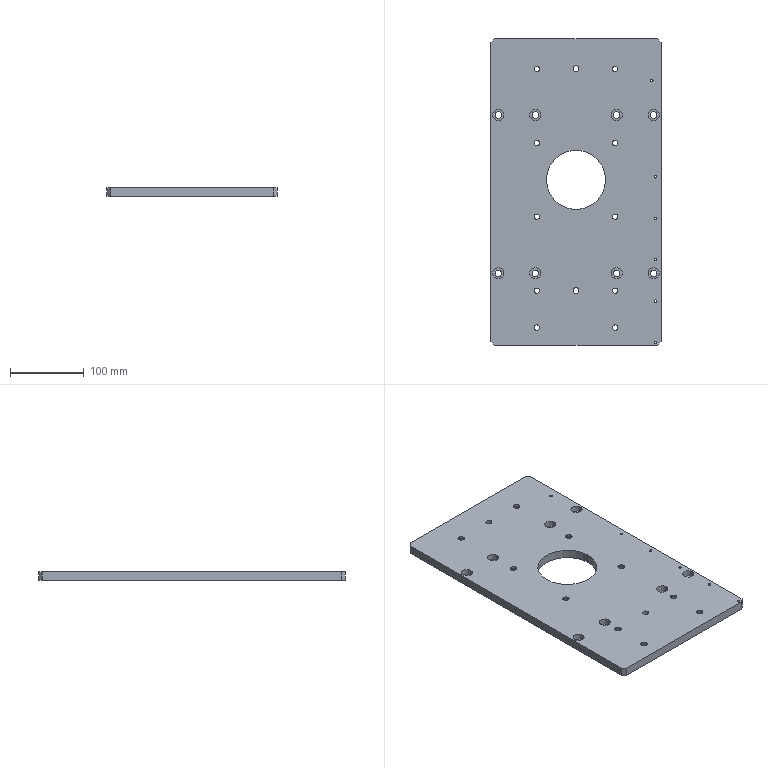Part | SolidWorks | features HoleWzd 5, Chamfer 1, Extrusion 1, ICE 1 | 1 solid | 138 faces | box 230 x 415 x 12 mm | volume 1051466 mm3 | cylinder 90 | plane 28 | cone 20 | commonest cylinder face diameters 9 x36 15 x36 3.3 x12 8 x4 80 x2